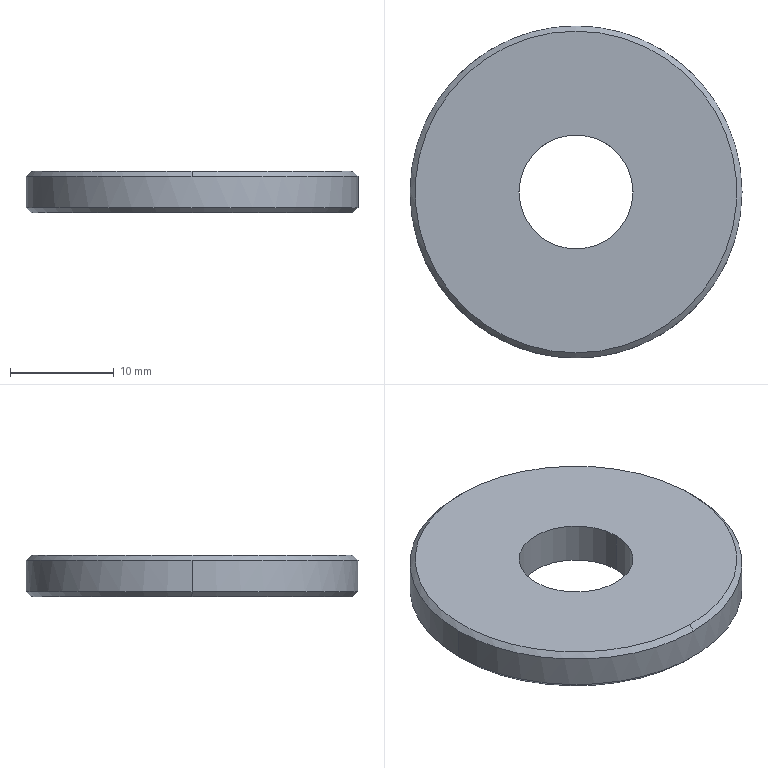Part | STEP file | 1 solid | 10 faces | box 32 x 32 x 4 mm | volume 2812 mm3 | cone 4 | cylinder 4 | plane 2 | commonest cylinder face diameters 11 x2 32 x2
STEP:
#1=CARTESIAN_POINT('',(0.,0.,0.));
#2=DIRECTION('',(0.,0.,1.));
#3=DIRECTION('',(1.,0.,0.));
#4=AXIS2_PLACEMENT_3D('',#1,#2,#3);
#5=CARTESIAN_POINT('',(0.,-15.5,4.));
#6=VERTEX_POINT('',#5);
#7=CARTESIAN_POINT('',(0.,-16.,3.5));
#8=VERTEX_POINT('',#7);
#9=CARTESIAN_POINT('',(0.,-16.,3.5));
#10=DIRECTION('',(0.,-0.7071,-0.7071));
#11=VECTOR('',#10,1.);
#12=LINE('',#9,#11);
#13=CARTESIAN_POINT('',(0.,0.,3.5));
#14=DIRECTION('',(0.,0.,-1.));
#15=DIRECTION('',(0.,1.,0.));
#16=AXIS2_PLACEMENT_3D('',#13,#14,#15);
#17=CONICAL_SURFACE('',#16,16.,0.7854);
#18=CARTESIAN_POINT('',(3.142,0.));
#19=DIRECTION('',(0.,1.));
#20=VECTOR('',#19,1.);
#21=LINE('',#18,#20);
#22=(GEOMETRIC_REPRESENTATION_CONTEXT(2)PARAMETRIC_REPRESENTATION_CONTEXT()REPRESENTATION_CONTEXT('',''));
#23=DEFINITIONAL_REPRESENTATION('',(#21),#22);
#24=PCURVE('',#17,#23);
#25=CARTESIAN_POINT('',(0.,0.,3.5));
#26=DIRECTION('',(0.,0.,-1.));
#27=DIRECTION('',(0.,1.,0.));
#28=AXIS2_PLACEMENT_3D('',#25,#26,#27);
#29=CONICAL_SURFACE('',#28,16.,0.7854);
#30=CARTESIAN_POINT('',(3.142,0.));
#31=DIRECTION('',(0.,1.));
#32=VECTOR('',#31,1.);
#33=LINE('',#30,#32);
#34=(GEOMETRIC_REPRESENTATION_CONTEXT(2)PARAMETRIC_REPRESENTATION_CONTEXT()REPRESENTATION_CONTEXT('',''));
#35=DEFINITIONAL_REPRESENTATION('',(#33),#34);
#36=PCURVE('',#29,#35);
#37=SURFACE_CURVE('',#12,(#24,#36),.PCURVE_S1.);
#38=EDGE_CURVE('',#6,#8,#37,.T.);
#39=ORIENTED_EDGE('',*,*,#38,.F.);
#40=CARTESIAN_POINT('',(0.,15.5,4.));
#41=VERTEX_POINT('',#40);
#42=CARTESIAN_POINT('',(0.,0.,4.));
#43=DIRECTION('',(0.,0.,1.));
#44=DIRECTION('',(0.,1.,0.));
#45=AXIS2_PLACEMENT_3D('',#42,#43,#44);
#46=CIRCLE('',#45,15.5);
#47=CARTESIAN_POINT('',(6.283,-0.5));
#48=DIRECTION('',(-1.,0.));
#49=VECTOR('',#48,1.);
#50=LINE('',#47,#49);
#51=(GEOMETRIC_REPRESENTATION_CONTEXT(2)PARAMETRIC_REPRESENTATION_CONTEXT()REPRESENTATION_CONTEXT('',''));
#52=DEFINITIONAL_REPRESENTATION('',(#50),#51);
#53=PCURVE('',#17,#52);
#54=CARTESIAN_POINT('',(0.,0.,4.));
#55=DIRECTION('',(0.,0.,1.));
#56=DIRECTION('',(1.,0.,0.));
#57=AXIS2_PLACEMENT_3D('',#54,#55,#56);
#58=PLANE('',#57);
#59=CARTESIAN_POINT('',(0.,0.));
#60=DIRECTION('',(0.,1.));
#61=AXIS2_PLACEMENT_2D('',#59,#60);
#62=CIRCLE('',#61,15.5);
#63=(GEOMETRIC_REPRESENTATION_CONTEXT(2)PARAMETRIC_REPRESENTATION_CONTEXT()REPRESENTATION_CONTEXT('',''));
#64=DEFINITIONAL_REPRESENTATION('',(#62),#63);
#65=PCURVE('',#58,#64);
#66=SURFACE_CURVE('',#46,(#53,#65),.PCURVE_S1.);
#67=EDGE_CURVE('',#41,#6,#66,.T.);
#68=ORIENTED_EDGE('',*,*,#67,.F.);
#69=CARTESIAN_POINT('',(0.,16.,3.5));
#70=VERTEX_POINT('',#69);
#71=CARTESIAN_POINT('',(0.,16.,3.5));
#72=DIRECTION('',(0.,0.7071,-0.7071));
#73=VECTOR('',#72,1.);
#74=LINE('',#71,#73);
#75=CARTESIAN_POINT('',(6.283,0.));
#76=DIRECTION('',(0.,1.));
#77=VECTOR('',#76,1.);
#78=LINE('',#75,#77);
#79=(GEOMETRIC_REPRESENTATION_CONTEXT(2)PARAMETRIC_REPRESENTATION_CONTEXT()REPRESENTATION_CONTEXT('',''));
#80=DEFINITIONAL_REPRESENTATION('',(#78),#79);
#81=PCURVE('',#17,#80);
#82=CARTESIAN_POINT('',(0.,0.));
#83=DIRECTION('',(0.,1.));
#84=VECTOR('',#83,1.);
#85=LINE('',#82,#84);
#86=(GEOMETRIC_REPRESENTATION_CONTEXT(2)PARAMETRIC_REPRESENTATION_CONTEXT()REPRESENTATION_CONTEXT('',''));
#87=DEFINITIONAL_REPRESENTATION('',(#85),#86);
#88=PCURVE('',#29,#87);
#89=SURFACE_CURVE('',#74,(#81,#88),.PCURVE_S1.);
#90=EDGE_CURVE('',#41,#70,#89,.T.);
#91=ORIENTED_EDGE('',*,*,#90,.T.);
#92=CARTESIAN_POINT('',(-16.,0.,3.5));
#93=VERTEX_POINT('',#92);
#94=CARTESIAN_POINT('',(0.,0.,3.5));
#95=DIRECTION('',(0.,0.,-1.));
#96=DIRECTION('',(-1.,0.,0.));
#97=AXIS2_PLACEMENT_3D('',#94,#95,#96);
#98=CIRCLE('',#97,16.);
#99=CARTESIAN_POINT('',(4.712,0.));
#100=DIRECTION('',(1.,0.));
#101=VECTOR('',#100,1.);
#102=LINE('',#99,#101);
#103=(GEOMETRIC_REPRESENTATION_CONTEXT(2)PARAMETRIC_REPRESENTATION_CONTEXT()REPRESENTATION_CONTEXT('',''));
#104=DEFINITIONAL_REPRESENTATION('',(#102),#103);
#105=PCURVE('',#17,#104);
#106=CARTESIAN_POINT('',(0.,0.,4.));
#107=DIRECTION('',(0.,0.,-1.));
#108=DIRECTION('',(-1.,0.,0.));
#109=AXIS2_PLACEMENT_3D('',#106,#107,#108);
#110=CYLINDRICAL_SURFACE('',#109,16.);
#111=CARTESIAN_POINT('',(0.,0.5));
#112=DIRECTION('',(1.,0.));
#113=VECTOR('',#112,1.);
#114=LINE('',#111,#113);
#115=(GEOMETRIC_REPRESENTATION_CONTEXT(2)PARAMETRIC_REPRESENTATION_CONTEXT()REPRESENTATION_CONTEXT('',''));
#116=DEFINITIONAL_REPRESENTATION('',(#114),#115);
#117=PCURVE('',#110,#116);
#118=SURFACE_CURVE('',#98,(#105,#117),.PCURVE_S1.);
#119=EDGE_CURVE('',#93,#70,#118,.T.);
#120=ORIENTED_EDGE('',*,*,#119,.F.);
#121=CARTESIAN_POINT('',(0.,0.,3.5));
#122=DIRECTION('',(0.,0.,-1.));
#123=DIRECTION('',(-1.,0.,0.));
#124=AXIS2_PLACEMENT_3D('',#121,#122,#123);
#125=CIRCLE('',#124,16.);
#126=CARTESIAN_POINT('',(-1.571,0.));
#127=DIRECTION('',(1.,0.));
#128=VECTOR('',#127,1.);
#129=LINE('',#126,#128);
#130=(GEOMETRIC_REPRESENTATION_CONTEXT(2)PARAMETRIC_REPRESENTATION_CONTEXT()REPRESENTATION_CONTEXT('',''));
#131=DEFINITIONAL_REPRESENTATION('',(#129),#130);
#132=PCURVE('',#17,#131);
#133=CARTESIAN_POINT('',(0.,0.,4.));
#134=DIRECTION('',(0.,0.,-1.));
#135=DIRECTION('',(-1.,0.,0.));
#136=AXIS2_PLACEMENT_3D('',#133,#134,#135);
#137=CYLINDRICAL_SURFACE('',#136,16.);
#138=CARTESIAN_POINT('',(0.,0.5));
#139=DIRECTION('',(1.,0.));
#140=VECTOR('',#139,1.);
#141=LINE('',#138,#140);
#142=(GEOMETRIC_REPRESENTATION_CONTEXT(2)PARAMETRIC_REPRESENTATION_CONTEXT()REPRESENTATION_CONTEXT('',''));
#143=DEFINITIONAL_REPRESENTATION('',(#141),#142);
#144=PCURVE('',#137,#143);
#145=SURFACE_CURVE('',#125,(#132,#144),.PCURVE_S1.);
#146=EDGE_CURVE('',#8,#93,#145,.T.);
#147=ORIENTED_EDGE('',*,*,#146,.F.);
#148=EDGE_LOOP('',(#39,#68,#91,#120,#147));
#149=FACE_BOUND('',#148,.T.);
#150=ADVANCED_FACE('',(#149),#17,.T.);
#151=CARTESIAN_POINT('',(16.,0.,3.5));
#152=VERTEX_POINT('',#151);
#153=CARTESIAN_POINT('',(16.,0.,0.5));
#154=VERTEX_POINT('',#153);
#155=CARTESIAN_POINT('',(16.,0.,4.));
#156=DIRECTION('',(0.,0.,-1.));
#157=VECTOR('',#156,1.);
#158=LINE('',#155,#157);
#159=CARTESIAN_POINT('',(3.142,0.));
#160=DIRECTION('',(0.,1.));
#161=VECTOR('',#160,1.);
#162=LINE('',#159,#161);
#163=(GEOMETRIC_REPRESENTATION_CONTEXT(2)PARAMETRIC_REPRESENTATION_CONTEXT()REPRESENTATION_CONTEXT('',''));
#164=DEFINITIONAL_REPRESENTATION('',(#162),#163);
#165=PCURVE('',#137,#164);
#166=CARTESIAN_POINT('',(3.142,0.));
#167=DIRECTION('',(0.,1.));
#168=VECTOR('',#167,1.);
#169=LINE('',#166,#168);
#170=(GEOMETRIC_REPRESENTATION_CONTEXT(2)PARAMETRIC_REPRESENTATION_CONTEXT()REPRESENTATION_CONTEXT('',''));
#171=DEFINITIONAL_REPRESENTATION('',(#169),#170);
#172=PCURVE('',#110,#171);
#173=SURFACE_CURVE('',#158,(#165,#172),.PCURVE_S1.);
#174=EDGE_CURVE('',#152,#154,#173,.T.);
#175=ORIENTED_EDGE('',*,*,#174,.F.);
#176=CARTESIAN_POINT('',(0.,0.,3.5));
#177=DIRECTION('',(0.,0.,-1.));
#178=DIRECTION('',(-1.,0.,0.));
#179=AXIS2_PLACEMENT_3D('',#176,#177,#178);
#180=CIRCLE('',#179,16.);
#181=CARTESIAN_POINT('',(0.,0.5));
#182=DIRECTION('',(1.,0.));
#183=VECTOR('',#182,1.);
#184=LINE('',#181,#183);
#185=(GEOMETRIC_REPRESENTATION_CONTEXT(2)PARAMETRIC_REPRESENTATION_CONTEXT()REPRESENTATION_CONTEXT('',''));
#186=DEFINITIONAL_REPRESENTATION('',(#184),#185);
#187=PCURVE('',#137,#186);
#188=CARTESIAN_POINT('',(-1.571,0.));
#189=DIRECTION('',(1.,0.));
#190=VECTOR('',#189,1.);
#191=LINE('',#188,#190);
#192=(GEOMETRIC_REPRESENTATION_CONTEXT(2)PARAMETRIC_REPRESENTATION_CONTEXT()REPRESENTATION_CONTEXT('',''));
#193=DEFINITIONAL_REPRESENTATION('',(#191),#192);
#194=PCURVE('',#29,#193);
#195=SURFACE_CURVE('',#180,(#187,#194),.PCURVE_S1.);
#196=EDGE_CURVE('',#152,#8,#195,.T.);
#197=ORIENTED_EDGE('',*,*,#196,.T.);
#198=ORIENTED_EDGE('',*,*,#146,.T.);
#199=CARTESIAN_POINT('',(-16.,0.,0.5));
#200=VERTEX_POINT('',#199);
#201=CARTESIAN_POINT('',(-16.,0.,4.));
#202=DIRECTION('',(0.,0.,-1.));
#203=VECTOR('',#202,1.);
#204=LINE('',#201,#203);
#205=CARTESIAN_POINT('',(6.283,0.));
#206=DIRECTION('',(0.,1.));
#207=VECTOR('',#206,1.);
#208=LINE('',#205,#207);
#209=(GEOMETRIC_REPRESENTATION_CONTEXT(2)PARAMETRIC_REPRESENTATION_CONTEXT()REPRESENTATION_CONTEXT('',''));
#210=DEFINITIONAL_REPRESENTATION('',(#208),#209);
#211=PCURVE('',#137,#210);
#212=CARTESIAN_POINT('',(0.,0.));
#213=DIRECTION('',(0.,1.));
#214=VECTOR('',#213,1.);
#215=LINE('',#212,#214);
#216=(GEOMETRIC_REPRESENTATION_CONTEXT(2)PARAMETRIC_REPRESENTATION_CONTEXT()REPRESENTATION_CONTEXT('',''));
#217=DEFINITIONAL_REPRESENTATION('',(#215),#216);
#218=PCURVE('',#110,#217);
#219=SURFACE_CURVE('',#204,(#211,#218),.PCURVE_S1.);
#220=EDGE_CURVE('',#93,#200,#219,.T.);
#221=ORIENTED_EDGE('',*,*,#220,.T.);
#222=CARTESIAN_POINT('',(0.,0.,0.5));
#223=DIRECTION('',(0.,0.,-1.));
#224=DIRECTION('',(1.,0.,0.));
#225=AXIS2_PLACEMENT_3D('',#222,#223,#224);
#226=CIRCLE('',#225,16.);
#227=CARTESIAN_POINT('',(3.142,3.5));
#228=DIRECTION('',(1.,0.));
#229=VECTOR('',#228,1.);
#230=LINE('',#227,#229);
#231=(GEOMETRIC_REPRESENTATION_CONTEXT(2)PARAMETRIC_REPRESENTATION_CONTEXT()REPRESENTATION_CONTEXT('',''));
#232=DEFINITIONAL_REPRESENTATION('',(#230),#231);
#233=PCURVE('',#137,#232);
#234=CARTESIAN_POINT('',(0.,0.,0.5));
#235=DIRECTION('',(0.,0.,1.));
#236=DIRECTION('',(1.,0.,0.));
#237=AXIS2_PLACEMENT_3D('',#234,#235,#236);
#238=CONICAL_SURFACE('',#237,16.,0.7854);
#239=CARTESIAN_POINT('',(6.283,0.));
#240=DIRECTION('',(-1.,0.));
#241=VECTOR('',#240,1.);
#242=LINE('',#239,#241);
#243=(GEOMETRIC_REPRESENTATION_CONTEXT(2)PARAMETRIC_REPRESENTATION_CONTEXT()REPRESENTATION_CONTEXT('',''));
#244=DEFINITIONAL_REPRESENTATION('',(#242),#243);
#245=PCURVE('',#238,#244);
#246=SURFACE_CURVE('',#226,(#233,#245),.PCURVE_S1.);
#247=EDGE_CURVE('',#154,#200,#246,.T.);
#248=ORIENTED_EDGE('',*,*,#247,.F.);
#249=EDGE_LOOP('',(#175,#197,#198,#221,#248));
#250=FACE_BOUND('',#249,.T.);
#251=ADVANCED_FACE('',(#250),#137,.T.);
#252=CARTESIAN_POINT('',(5.5,0.,4.));
#253=VERTEX_POINT('',#252);
#254=CARTESIAN_POINT('',(-5.5,0.,4.));
#255=VERTEX_POINT('',#254);
#256=CARTESIAN_POINT('',(0.,0.,4.));
#257=DIRECTION('',(0.,0.,-1.));
#258=DIRECTION('',(1.,0.,0.));
#259=AXIS2_PLACEMENT_3D('',#256,#257,#258);
#260=CIRCLE('',#259,5.5);
#261=CARTESIAN_POINT('',(5.5,0.));
#262=CARTESIAN_POINT('',(5.5,-9.526));
#263=CARTESIAN_POINT('',(-2.75,-4.763));
#264=CARTESIAN_POINT('',(-11.,0.));
#265=CARTESIAN_POINT('',(-2.75,4.763));
#266=CARTESIAN_POINT('',(5.5,9.526));
#267=CARTESIAN_POINT('',(5.5,0.));
#268=(BOUNDED_CURVE()B_SPLINE_CURVE(2,(#261,#262,#263,#264,#265,#266,#267),.UNSPECIFIED.,.T.,.F.)B_SPLINE_CURVE_WITH_KNOTS((1,2,2,2,2,1),(-2.094,0.,2.094,4.189,6.283,8.378),.UNSPECIFIED.)CURVE()GEOMETRIC_REPRESENTATION_ITEM()RATIONAL_B_SPLINE_CURVE((1.,0.5,1.,0.5,1.,0.5,1.))REPRESENTATION_ITEM(''));
#269=(GEOMETRIC_REPRESENTATION_CONTEXT(2)PARAMETRIC_REPRESENTATION_CONTEXT()REPRESENTATION_CONTEXT('',''));
#270=DEFINITIONAL_REPRESENTATION('',(#268),#269);
#271=PCURVE('',#58,#270);
#272=CARTESIAN_POINT('',(0.,0.,0.));
#273=DIRECTION('',(0.,0.,1.));
#274=DIRECTION('',(1.,0.,0.));
#275=AXIS2_PLACEMENT_3D('',#272,#273,#274);
#276=CYLINDRICAL_SURFACE('',#275,5.5);
#277=CARTESIAN_POINT('',(6.283,4.));
#278=DIRECTION('',(-1.,0.));
#279=VECTOR('',#278,1.);
#280=LINE('',#277,#279);
#281=(GEOMETRIC_REPRESENTATION_CONTEXT(2)PARAMETRIC_REPRESENTATION_CONTEXT()REPRESENTATION_CONTEXT('',''));
#282=DEFINITIONAL_REPRESENTATION('',(#280),#281);
#283=PCURVE('',#276,#282);
#284=SURFACE_CURVE('',#260,(#271,#283),.PCURVE_S1.);
#285=EDGE_CURVE('',#253,#255,#284,.T.);
#286=ORIENTED_EDGE('',*,*,#285,.T.);
#287=CARTESIAN_POINT('',(0.,0.,4.));
#288=DIRECTION('',(0.,0.,-1.));
#289=DIRECTION('',(1.,0.,0.));
#290=AXIS2_PLACEMENT_3D('',#287,#288,#289);
#291=CIRCLE('',#290,5.5);
#292=CARTESIAN_POINT('',(5.5,0.));
#293=CARTESIAN_POINT('',(5.5,-9.526));
#294=CARTESIAN_POINT('',(-2.75,-4.763));
#295=CARTESIAN_POINT('',(-11.,0.));
#296=CARTESIAN_POINT('',(-2.75,4.763));
#297=CARTESIAN_POINT('',(5.5,9.526));
#298=CARTESIAN_POINT('',(5.5,0.));
#299=(BOUNDED_CURVE()B_SPLINE_CURVE(2,(#292,#293,#294,#295,#296,#297,#298),.UNSPECIFIED.,.T.,.F.)B_SPLINE_CURVE_WITH_KNOTS((1,2,2,2,2,1),(-2.094,0.,2.094,4.189,6.283,8.378),.UNSPECIFIED.)CURVE()GEOMETRIC_REPRESENTATION_ITEM()RATIONAL_B_SPLINE_CURVE((1.,0.5,1.,0.5,1.,0.5,1.))REPRESENTATION_ITEM(''));
#300=(GEOMETRIC_REPRESENTATION_CONTEXT(2)PARAMETRIC_REPRESENTATION_CONTEXT()REPRESENTATION_CONTEXT('',''));
#301=DEFINITIONAL_REPRESENTATION('',(#299),#300);
#302=PCURVE('',#58,#301);
#303=CARTESIAN_POINT('',(0.,0.,0.));
#304=DIRECTION('',(0.,0.,1.));
#305=DIRECTION('',(1.,0.,0.));
#306=AXIS2_PLACEMENT_3D('',#303,#304,#305);
#307=CYLINDRICAL_SURFACE('',#306,5.5);
#308=CARTESIAN_POINT('',(6.283,4.));
#309=DIRECTION('',(-1.,0.));
#310=VECTOR('',#309,1.);
#311=LINE('',#308,#310);
#312=(GEOMETRIC_REPRESENTATION_CONTEXT(2)PARAMETRIC_REPRESENTATION_CONTEXT()REPRESENTATION_CONTEXT('',''));
#313=DEFINITIONAL_REPRESENTATION('',(#311),#312);
#314=PCURVE('',#307,#313);
#315=SURFACE_CURVE('',#291,(#302,#314),.PCURVE_S1.);
#316=EDGE_CURVE('',#255,#253,#315,.T.);
#317=ORIENTED_EDGE('',*,*,#316,.T.);
#318=EDGE_LOOP('',(#286,#317));
#319=FACE_BOUND('',#318,.T.);
#320=ORIENTED_EDGE('',*,*,#67,.T.);
#321=CARTESIAN_POINT('',(0.,0.,4.));
#322=DIRECTION('',(0.,0.,1.));
#323=DIRECTION('',(0.,1.,0.));
#324=AXIS2_PLACEMENT_3D('',#321,#322,#323);
#325=CIRCLE('',#324,15.5);
#326=CARTESIAN_POINT('',(0.,0.));
#327=DIRECTION('',(0.,1.));
#328=AXIS2_PLACEMENT_2D('',#326,#327);
#329=CIRCLE('',#328,15.5);
#330=(GEOMETRIC_REPRESENTATION_CONTEXT(2)PARAMETRIC_REPRESENTATION_CONTEXT()REPRESENTATION_CONTEXT('',''));
#331=DEFINITIONAL_REPRESENTATION('',(#329),#330);
#332=PCURVE('',#58,#331);
#333=CARTESIAN_POINT('',(6.283,-0.5));
#334=DIRECTION('',(-1.,0.));
#335=VECTOR('',#334,1.);
#336=LINE('',#333,#335);
#337=(GEOMETRIC_REPRESENTATION_CONTEXT(2)PARAMETRIC_REPRESENTATION_CONTEXT()REPRESENTATION_CONTEXT('',''));
#338=DEFINITIONAL_REPRESENTATION('',(#336),#337);
#339=PCURVE('',#29,#338);
#340=SURFACE_CURVE('',#325,(#332,#339),.PCURVE_S1.);
#341=EDGE_CURVE('',#6,#41,#340,.T.);
#342=ORIENTED_EDGE('',*,*,#341,.T.);
#343=EDGE_LOOP('',(#320,#342));
#344=FACE_BOUND('',#343,.T.);
#345=ADVANCED_FACE('',(#319,#344),#58,.T.);
#346=CARTESIAN_POINT('',(-15.5,0.,0.));
#347=VERTEX_POINT('',#346);
#348=CARTESIAN_POINT('',(-16.,0.,0.5));
#349=DIRECTION('',(-0.7071,0.,0.7071));
#350=VECTOR('',#349,1.);
#351=LINE('',#348,#350);
#352=CARTESIAN_POINT('',(3.142,0.));
#353=DIRECTION('',(0.,1.));
#354=VECTOR('',#353,1.);
#355=LINE('',#352,#354);
#356=(GEOMETRIC_REPRESENTATION_CONTEXT(2)PARAMETRIC_REPRESENTATION_CONTEXT()REPRESENTATION_CONTEXT('',''));
#357=DEFINITIONAL_REPRESENTATION('',(#355),#356);
#358=PCURVE('',#238,#357);
#359=CARTESIAN_POINT('',(0.,0.,0.5));
#360=DIRECTION('',(0.,0.,1.));
#361=DIRECTION('',(1.,0.,0.));
#362=AXIS2_PLACEMENT_3D('',#359,#360,#361);
#363=CONICAL_SURFACE('',#362,16.,0.7854);
#364=CARTESIAN_POINT('',(3.142,0.));
#365=DIRECTION('',(0.,1.));
#366=VECTOR('',#365,1.);
#367=LINE('',#364,#366);
#368=(GEOMETRIC_REPRESENTATION_CONTEXT(2)PARAMETRIC_REPRESENTATION_CONTEXT()REPRESENTATION_CONTEXT('',''));
#369=DEFINITIONAL_REPRESENTATION('',(#367),#368);
#370=PCURVE('',#363,#369);
#371=SURFACE_CURVE('',#351,(#358,#370),.PCURVE_S1.);
#372=EDGE_CURVE('',#347,#200,#371,.T.);
#373=ORIENTED_EDGE('',*,*,#372,.F.);
#374=CARTESIAN_POINT('',(15.5,0.,0.));
#375=VERTEX_POINT('',#374);
#376=CARTESIAN_POINT('',(0.,0.,0.));
#377=DIRECTION('',(0.,0.,1.));
#378=DIRECTION('',(1.,0.,0.));
#379=AXIS2_PLACEMENT_3D('',#376,#377,#378);
#380=CIRCLE('',#379,15.5);
#381=CARTESIAN_POINT('',(0.,-0.5));
#382=DIRECTION('',(1.,0.));
#383=VECTOR('',#382,1.);
#384=LINE('',#381,#383);
#385=(GEOMETRIC_REPRESENTATION_CONTEXT(2)PARAMETRIC_REPRESENTATION_CONTEXT()REPRESENTATION_CONTEXT('',''));
#386=DEFINITIONAL_REPRESENTATION('',(#384),#385);
#387=PCURVE('',#238,#386);
#388=CARTESIAN_POINT('',(0.,0.,0.));
#389=DIRECTION('',(0.,0.,1.));
#390=DIRECTION('',(1.,0.,0.));
#391=AXIS2_PLACEMENT_3D('',#388,#389,#390);
#392=PLANE('',#391);
#393=CARTESIAN_POINT('',(0.,0.));
#394=DIRECTION('',(1.,0.));
#395=AXIS2_PLACEMENT_2D('',#393,#394);
#396=CIRCLE('',#395,15.5);
#397=(GEOMETRIC_REPRESENTATION_CONTEXT(2)PARAMETRIC_REPRESENTATION_CONTEXT()REPRESENTATION_CONTEXT('',''));
#398=DEFINITIONAL_REPRESENTATION('',(#396),#397);
#399=PCURVE('',#392,#398);
#400=SURFACE_CURVE('',#380,(#387,#399),.PCURVE_S1.);
#401=EDGE_CURVE('',#347,#375,#400,.T.);
#402=ORIENTED_EDGE('',*,*,#401,.T.);
#403=CARTESIAN_POINT('',(16.,0.,0.5));
#404=DIRECTION('',(0.7071,0.,0.7071));
#405=VECTOR('',#404,1.);
#406=LINE('',#403,#405);
#407=CARTESIAN_POINT('',(6.283,0.));
#408=DIRECTION('',(0.,1.));
#409=VECTOR('',#408,1.);
#410=LINE('',#407,#409);
#411=(GEOMETRIC_REPRESENTATION_CONTEXT(2)PARAMETRIC_REPRESENTATION_CONTEXT()REPRESENTATION_CONTEXT('',''));
#412=DEFINITIONAL_REPRESENTATION('',(#410),#411);
#413=PCURVE('',#238,#412);
#414=CARTESIAN_POINT('',(0.,0.));
#415=DIRECTION('',(0.,1.));
#416=VECTOR('',#415,1.);
#417=LINE('',#414,#416);
#418=(GEOMETRIC_REPRESENTATION_CONTEXT(2)PARAMETRIC_REPRESENTATION_CONTEXT()REPRESENTATION_CONTEXT('',''));
#419=DEFINITIONAL_REPRESENTATION('',(#417),#418);
#420=PCURVE('',#363,#419);
#421=SURFACE_CURVE('',#406,(#413,#420),.PCURVE_S1.);
#422=EDGE_CURVE('',#375,#154,#421,.T.);
#423=ORIENTED_EDGE('',*,*,#422,.T.);
#424=ORIENTED_EDGE('',*,*,#247,.T.);
#425=EDGE_LOOP('',(#373,#402,#423,#424));
#426=FACE_BOUND('',#425,.T.);
#427=ADVANCED_FACE('',(#426),#238,.T.);
#428=ORIENTED_EDGE('',*,*,#316,.T.);
#429=CARTESIAN_POINT('',(5.5,0.,0.));
#430=VERTEX_POINT('',#429);
#431=CARTESIAN_POINT('',(5.5,0.,0.));
#432=DIRECTION('',(0.,0.,1.));
#433=VECTOR('',#432,1.);
#434=LINE('',#431,#433);
#435=CARTESIAN_POINT('',(0.,0.));
#436=DIRECTION('',(0.,1.));
#437=VECTOR('',#436,1.);
#438=LINE('',#435,#437);
#439=(GEOMETRIC_REPRESENTATION_CONTEXT(2)PARAMETRIC_REPRESENTATION_CONTEXT()REPRESENTATION_CONTEXT('',''));
#440=DEFINITIONAL_REPRESENTATION('',(#438),#439);
#441=PCURVE('',#307,#440);
#442=CARTESIAN_POINT('',(6.283,0.));
#443=DIRECTION('',(0.,1.));
#444=VECTOR('',#443,1.);
#445=LINE('',#442,#444);
#446=(GEOMETRIC_REPRESENTATION_CONTEXT(2)PARAMETRIC_REPRESENTATION_CONTEXT()REPRESENTATION_CONTEXT('',''));
#447=DEFINITIONAL_REPRESENTATION('',(#445),#446);
#448=PCURVE('',#276,#447);
#449=SURFACE_CURVE('',#434,(#441,#448),.PCURVE_S1.);
#450=EDGE_CURVE('',#430,#253,#449,.T.);
#451=ORIENTED_EDGE('',*,*,#450,.F.);
#452=CARTESIAN_POINT('',(-5.5,0.,0.));
#453=VERTEX_POINT('',#452);
#454=CARTESIAN_POINT('',(0.,0.,0.));
#455=DIRECTION('',(0.,0.,-1.));
#456=DIRECTION('',(1.,0.,0.));
#457=AXIS2_PLACEMENT_3D('',#454,#455,#456);
#458=CIRCLE('',#457,5.5);
#459=CARTESIAN_POINT('',(6.283,0.));
#460=DIRECTION('',(-1.,0.));
#461=VECTOR('',#460,1.);
#462=LINE('',#459,#461);
#463=(GEOMETRIC_REPRESENTATION_CONTEXT(2)PARAMETRIC_REPRESENTATION_CONTEXT()REPRESENTATION_CONTEXT('',''));
#464=DEFINITIONAL_REPRESENTATION('',(#462),#463);
#465=PCURVE('',#307,#464);
#466=CARTESIAN_POINT('',(5.5,0.));
#467=CARTESIAN_POINT('',(5.5,-9.526));
#468=CARTESIAN_POINT('',(-2.75,-4.763));
#469=CARTESIAN_POINT('',(-11.,0.));
#470=CARTESIAN_POINT('',(-2.75,4.763));
#471=CARTESIAN_POINT('',(5.5,9.526));
#472=CARTESIAN_POINT('',(5.5,0.));
#473=(BOUNDED_CURVE()B_SPLINE_CURVE(2,(#466,#467,#468,#469,#470,#471,#472),.UNSPECIFIED.,.T.,.F.)B_SPLINE_CURVE_WITH_KNOTS((1,2,2,2,2,1),(-2.094,0.,2.094,4.189,6.283,8.378),.UNSPECIFIED.)CURVE()GEOMETRIC_REPRESENTATION_ITEM()RATIONAL_B_SPLINE_CURVE((1.,0.5,1.,0.5,1.,0.5,1.))REPRESENTATION_ITEM(''));
#474=(GEOMETRIC_REPRESENTATION_CONTEXT(2)PARAMETRIC_REPRESENTATION_CONTEXT()REPRESENTATION_CONTEXT('',''));
#475=DEFINITIONAL_REPRESENTATION('',(#473),#474);
#476=PCURVE('',#392,#475);
#477=SURFACE_CURVE('',#458,(#465,#476),.PCURVE_S1.);
#478=EDGE_CURVE('',#453,#430,#477,.T.);
#479=ORIENTED_EDGE('',*,*,#478,.F.);
#480=CARTESIAN_POINT('',(-5.5,0.,0.));
#481=DIRECTION('',(0.,0.,1.));
#482=VECTOR('',#481,1.);
#483=LINE('',#480,#482);
#484=CARTESIAN_POINT('',(3.142,0.));
#485=DIRECTION('',(0.,1.));
#486=VECTOR('',#485,1.);
#487=LINE('',#484,#486);
#488=(GEOMETRIC_REPRESENTATION_CONTEXT(2)PARAMETRIC_REPRESENTATION_CONTEXT()REPRESENTATION_CONTEXT('',''));
#489=DEFINITIONAL_REPRESENTATION('',(#487),#488);
#490=PCURVE('',#307,#489);
#491=CARTESIAN_POINT('',(3.142,0.));
#492=DIRECTION('',(0.,1.));
#493=VECTOR('',#492,1.);
#494=LINE('',#491,#493);
#495=(GEOMETRIC_REPRESENTATION_CONTEXT(2)PARAMETRIC_REPRESENTATION_CONTEXT()REPRESENTATION_CONTEXT('',''));
#496=DEFINITIONAL_REPRESENTATION('',(#494),#495);
#497=PCURVE('',#276,#496);
#498=SURFACE_CURVE('',#483,(#490,#497),.PCURVE_S1.);
#499=EDGE_CURVE('',#453,#255,#498,.T.);
#500=ORIENTED_EDGE('',*,*,#499,.T.);
#501=EDGE_LOOP('',(#428,#451,#479,#500));
#502=FACE_BOUND('',#501,.F.);
#503=ADVANCED_FACE('',(#502),#307,.F.);
#504=CARTESIAN_POINT('',(0.,0.,0.));
#505=DIRECTION('',(0.,0.,-1.));
#506=DIRECTION('',(1.,0.,0.));
#507=AXIS2_PLACEMENT_3D('',#504,#505,#506);
#508=CIRCLE('',#507,5.5);
#509=CARTESIAN_POINT('',(5.5,0.));
#510=CARTESIAN_POINT('',(5.5,-9.526));
#511=CARTESIAN_POINT('',(-2.75,-4.763));
#512=CARTESIAN_POINT('',(-11.,0.));
#513=CARTESIAN_POINT('',(-2.75,4.763));
#514=CARTESIAN_POINT('',(5.5,9.526));
#515=CARTESIAN_POINT('',(5.5,0.));
#516=(BOUNDED_CURVE()B_SPLINE_CURVE(2,(#509,#510,#511,#512,#513,#514,#515),.UNSPECIFIED.,.T.,.F.)B_SPLINE_CURVE_WITH_KNOTS((1,2,2,2,2,1),(-2.094,0.,2.094,4.189,6.283,8.378),.UNSPECIFIED.)CURVE()GEOMETRIC_REPRESENTATION_ITEM()RATIONAL_B_SPLINE_CURVE((1.,0.5,1.,0.5,1.,0.5,1.))REPRESENTATION_ITEM(''));
#517=(GEOMETRIC_REPRESENTATION_CONTEXT(2)PARAMETRIC_REPRESENTATION_CONTEXT()REPRESENTATION_CONTEXT('',''));
#518=DEFINITIONAL_REPRESENTATION('',(#516),#517);
#519=PCURVE('',#392,#518);
#520=CARTESIAN_POINT('',(6.283,0.));
#521=DIRECTION('',(-1.,0.));
#522=VECTOR('',#521,1.);
#523=LINE('',#520,#522);
#524=(GEOMETRIC_REPRESENTATION_CONTEXT(2)PARAMETRIC_REPRESENTATION_CONTEXT()REPRESENTATION_CONTEXT('',''));
#525=DEFINITIONAL_REPRESENTATION('',(#523),#524);
#526=PCURVE('',#276,#525);
#527=SURFACE_CURVE('',#508,(#519,#526),.PCURVE_S1.);
#528=EDGE_CURVE('',#430,#453,#527,.T.);
#529=ORIENTED_EDGE('',*,*,#528,.F.);
#530=ORIENTED_EDGE('',*,*,#478,.F.);
#531=EDGE_LOOP('',(#529,#530));
#532=FACE_BOUND('',#531,.T.);
#533=CARTESIAN_POINT('',(0.,0.,0.));
#534=DIRECTION('',(0.,0.,1.));
#535=DIRECTION('',(1.,0.,0.));
#536=AXIS2_PLACEMENT_3D('',#533,#534,#535);
#537=CIRCLE('',#536,15.5);
#538=CARTESIAN_POINT('',(0.,0.));
#539=DIRECTION('',(1.,0.));
#540=AXIS2_PLACEMENT_2D('',#538,#539);
#541=CIRCLE('',#540,15.5);
#542=(GEOMETRIC_REPRESENTATION_CONTEXT(2)PARAMETRIC_REPRESENTATION_CONTEXT()REPRESENTATION_CONTEXT('',''));
#543=DEFINITIONAL_REPRESENTATION('',(#541),#542);
#544=PCURVE('',#392,#543);
#545=CARTESIAN_POINT('',(0.,-0.5));
#546=DIRECTION('',(1.,0.));
#547=VECTOR('',#546,1.);
#548=LINE('',#545,#547);
#549=(GEOMETRIC_REPRESENTATION_CONTEXT(2)PARAMETRIC_REPRESENTATION_CONTEXT()REPRESENTATION_CONTEXT('',''));
#550=DEFINITIONAL_REPRESENTATION('',(#548),#549);
#551=PCURVE('',#363,#550);
#552=SURFACE_CURVE('',#537,(#544,#551),.PCURVE_S1.);
#553=EDGE_CURVE('',#375,#347,#552,.T.);
#554=ORIENTED_EDGE('',*,*,#553,.F.);
#555=ORIENTED_EDGE('',*,*,#401,.F.);
#556=EDGE_LOOP('',(#554,#555));
#557=FACE_BOUND('',#556,.T.);
#558=ADVANCED_FACE('',(#532,#557),#392,.F.);
#559=ORIENTED_EDGE('',*,*,#341,.F.);
#560=ORIENTED_EDGE('',*,*,#38,.T.);
#561=ORIENTED_EDGE('',*,*,#196,.F.);
#562=CARTESIAN_POINT('',(0.,0.,3.5));
#563=DIRECTION('',(0.,0.,-1.));
#564=DIRECTION('',(-1.,0.,0.));
#565=AXIS2_PLACEMENT_3D('',#562,#563,#564);
#566=CIRCLE('',#565,16.);
#567=CARTESIAN_POINT('',(-1.571,0.));
#568=DIRECTION('',(1.,0.));
#569=VECTOR('',#568,1.);
#570=LINE('',#567,#569);
#571=(GEOMETRIC_REPRESENTATION_CONTEXT(2)PARAMETRIC_REPRESENTATION_CONTEXT()REPRESENTATION_CONTEXT('',''));
#572=DEFINITIONAL_REPRESENTATION('',(#570),#571);
#573=PCURVE('',#29,#572);
#574=CARTESIAN_POINT('',(0.,0.5));
#575=DIRECTION('',(1.,0.));
#576=VECTOR('',#575,1.);
#577=LINE('',#574,#576);
#578=(GEOMETRIC_REPRESENTATION_CONTEXT(2)PARAMETRIC_REPRESENTATION_CONTEXT()REPRESENTATION_CONTEXT('',''));
#579=DEFINITIONAL_REPRESENTATION('',(#577),#578);
#580=PCURVE('',#110,#579);
#581=SURFACE_CURVE('',#566,(#573,#580),.PCURVE_S1.);
#582=EDGE_CURVE('',#70,#152,#581,.T.);
#583=ORIENTED_EDGE('',*,*,#582,.F.);
#584=ORIENTED_EDGE('',*,*,#90,.F.);
#585=EDGE_LOOP('',(#559,#560,#561,#583,#584));
#586=FACE_BOUND('',#585,.T.);
#587=ADVANCED_FACE('',(#586),#29,.T.);
#588=ORIENTED_EDGE('',*,*,#582,.T.);
#589=ORIENTED_EDGE('',*,*,#174,.T.);
#590=CARTESIAN_POINT('',(0.,0.,0.5));
#591=DIRECTION('',(0.,0.,-1.));
#592=DIRECTION('',(1.,0.,0.));
#593=AXIS2_PLACEMENT_3D('',#590,#591,#592);
#594=CIRCLE('',#593,16.);
#595=CARTESIAN_POINT('',(-3.142,3.5));
#596=DIRECTION('',(1.,0.));
#597=VECTOR('',#596,1.);
#598=LINE('',#595,#597);
#599=(GEOMETRIC_REPRESENTATION_CONTEXT(2)PARAMETRIC_REPRESENTATION_CONTEXT()REPRESENTATION_CONTEXT('',''));
#600=DEFINITIONAL_REPRESENTATION('',(#598),#599);
#601=PCURVE('',#110,#600);
#602=CARTESIAN_POINT('',(6.283,0.));
#603=DIRECTION('',(-1.,0.));
#604=VECTOR('',#603,1.);
#605=LINE('',#602,#604);
#606=(GEOMETRIC_REPRESENTATION_CONTEXT(2)PARAMETRIC_REPRESENTATION_CONTEXT()REPRESENTATION_CONTEXT('',''));
#607=DEFINITIONAL_REPRESENTATION('',(#605),#606);
#608=PCURVE('',#363,#607);
#609=SURFACE_CURVE('',#594,(#601,#608),.PCURVE_S1.);
#610=EDGE_CURVE('',#200,#154,#609,.T.);
#611=ORIENTED_EDGE('',*,*,#610,.F.);
#612=ORIENTED_EDGE('',*,*,#220,.F.);
#613=ORIENTED_EDGE('',*,*,#119,.T.);
#614=EDGE_LOOP('',(#588,#589,#611,#612,#613));
#615=FACE_BOUND('',#614,.T.);
#616=ADVANCED_FACE('',(#615),#110,.T.);
#617=ORIENTED_EDGE('',*,*,#553,.T.);
#618=ORIENTED_EDGE('',*,*,#372,.T.);
#619=ORIENTED_EDGE('',*,*,#610,.T.);
#620=ORIENTED_EDGE('',*,*,#422,.F.);
#621=EDGE_LOOP('',(#617,#618,#619,#620));
#622=FACE_BOUND('',#621,.T.);
#623=ADVANCED_FACE('',(#622),#363,.T.);
#624=ORIENTED_EDGE('',*,*,#450,.T.);
#625=ORIENTED_EDGE('',*,*,#285,.T.);
#626=ORIENTED_EDGE('',*,*,#499,.F.);
#627=ORIENTED_EDGE('',*,*,#528,.F.);
#628=EDGE_LOOP('',(#624,#625,#626,#627));
#629=FACE_BOUND('',#628,.F.);
#630=ADVANCED_FACE('',(#629),#276,.F.);
#631=CLOSED_SHELL('',(#150,#251,#345,#427,#503,#558,#587,#616,#623,#630));
#632=MANIFOLD_SOLID_BREP('',#631);
#633=(LENGTH_UNIT()NAMED_UNIT(*)SI_UNIT(.MILLI.,.METRE.));
#634=UNCERTAINTY_MEASURE_WITH_UNIT(LENGTH_MEASURE(0.0000001),#633,'','');
#635=(NAMED_UNIT(*)PLANE_ANGLE_UNIT()SI_UNIT($,.RADIAN.));
#636=(NAMED_UNIT(*)SI_UNIT($,.STERADIAN.)SOLID_ANGLE_UNIT());
#637=(GEOMETRIC_REPRESENTATION_CONTEXT(3)GLOBAL_UNCERTAINTY_ASSIGNED_CONTEXT((#634))GLOBAL_UNIT_ASSIGNED_CONTEXT((#633,#635,#636))REPRESENTATION_CONTEXT('',''));
#638=ADVANCED_BREP_SHAPE_REPRESENTATION('',(#4,#632),#637);